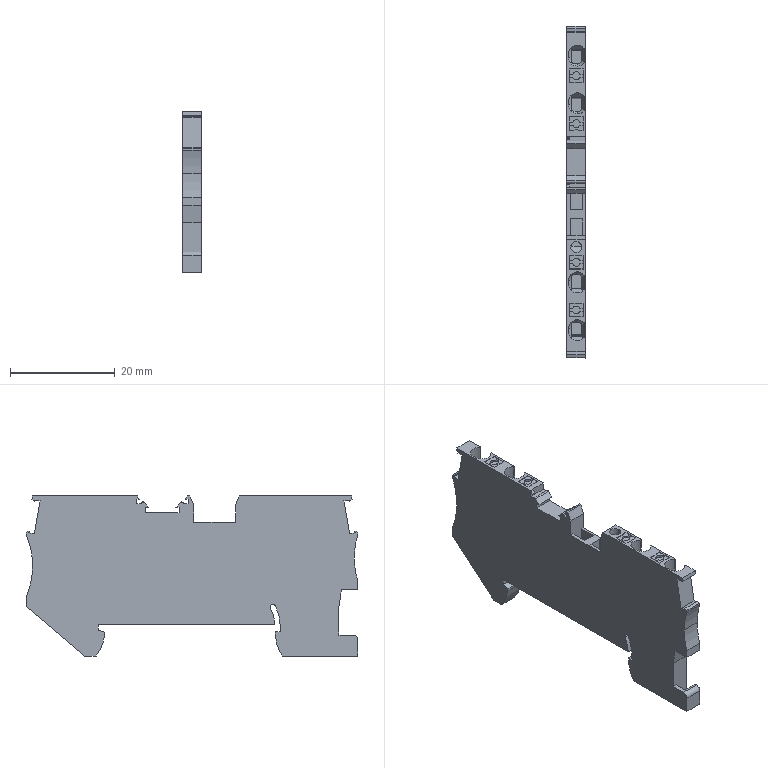Part | STEP file | Feed-through terminal block PT 1.5-S-QUATTRO | 1 solid | 270 faces | box 3.5 x 63.2 x 30.5 mm | volume 4808 mm3 | plane 210 | cylinder 54 | cone 6 | commonest cylinder face diameters 3.4 x12 1 x10 1.5 x10 1.6 x8 30 x3 0.6 x2